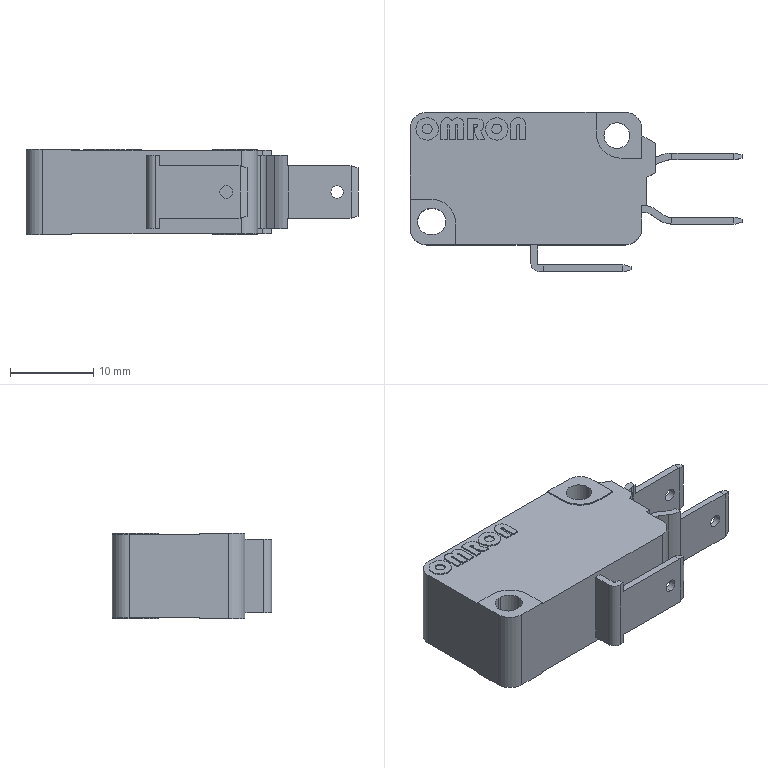Part | SolidWorks | features ICE 8, Chamfer 4, Extrusion 1, MirrorPattern 1 | 1 solid | 177 faces | box 39.8 x 19.1 x 10.3 mm | volume 4486 mm3 | plane 114 | spline 32 | cylinder 31 | commonest cylinder face diameters 1.5 x7 4 x7 3.1 x5 6 x4 1 x3 2.4 x2